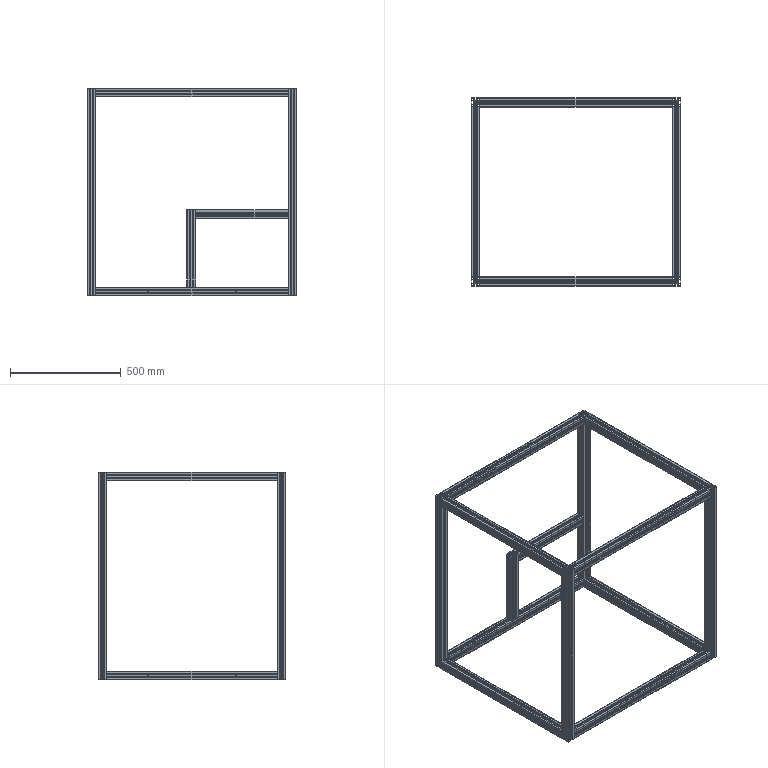Part | SolidWorks | features WeldCornerFeat 8, 3DProfileFeature 5, HoleWzd 4, ICE 1, WeldMemberFeat 1, WeldmentFeature 1 | 14 solids | 2182 faces | box 950 x 850 x 940 mm | volume 5673815 mm3 | plane 1713 | cylinder 469 | commonest cylinder face diameters 13.3 x293 12 x60 0.6 x56 6.8 x44 7 x16